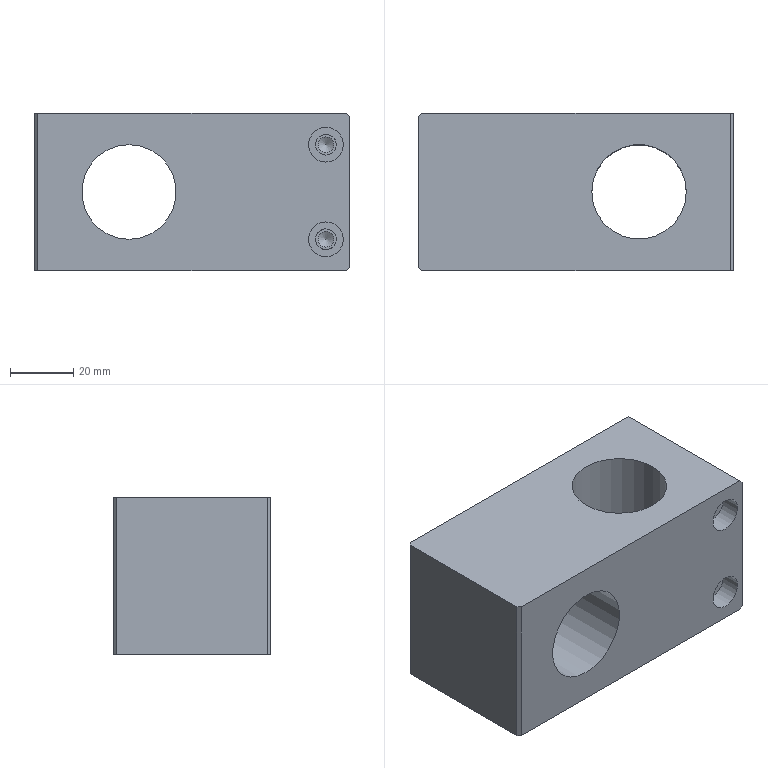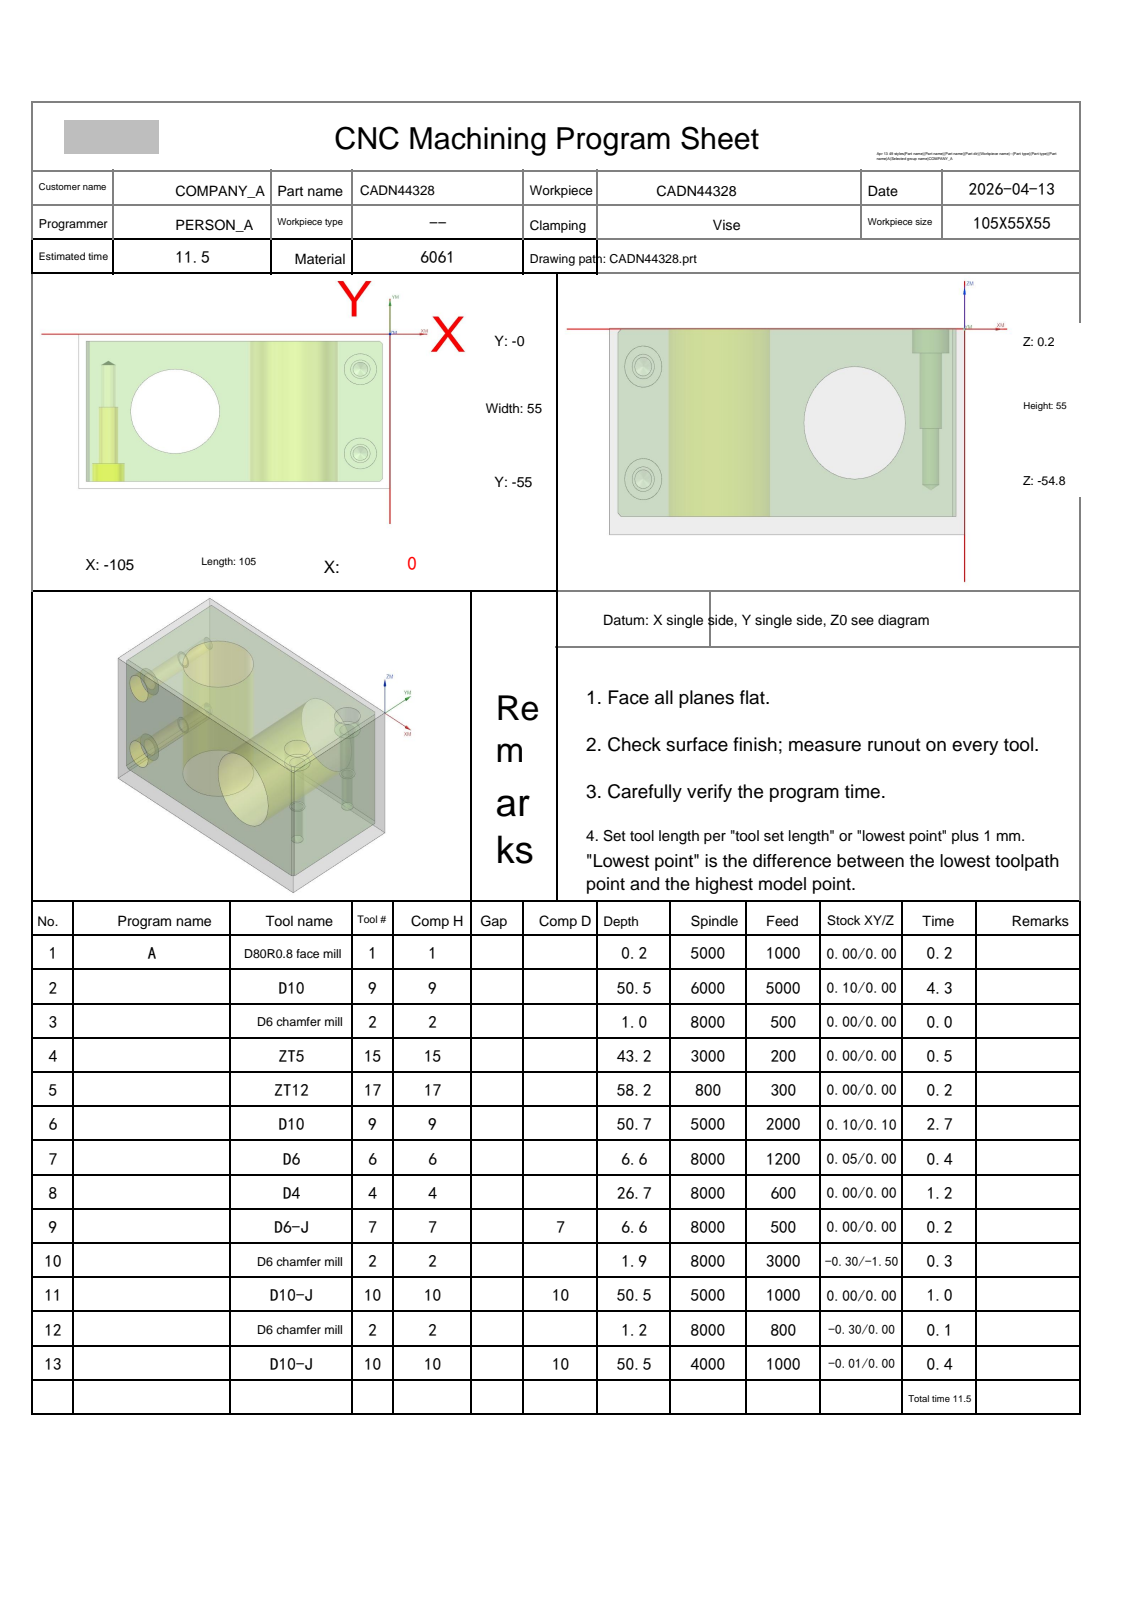NC program | NX | posted by the shop | part box 100 x 50 x 50 mm
Whole program, first 1102 of 1761 lines:
%
O0001
(Machine time: 14.12 MIN)
(===Total Tool:9===)
(T1=D80R0.8 face mill D=80. R=0.8 D- H01 Z=0.    )
(T9=D10 D=10. R=0. D- H09 Z=-50.5 )
(T2=D6 chamfer mill D=6. R=0. D- H02 Z=-1.7  )
(T15=ZT5 D=5. DR_a=118 D- H15 Z=-43.  )
(T17=ZT12 D=12. DR_a=118 D- H17 Z=-58.  )
(T6=D6 D=6. R=0. D- H06 Z=-6.4  )
(T4=D4 D=4. R=0. D- H04 Z=-26.5 )
(T7=D6-J D=6. R=0. D7 H07 Z=-6.4  )
(T10=D10-J D=10. R=0. D10 H10 Z=-50.3 )
G80 G90 G17 G49 G40
G91 G28 Z0
M01
N1 T01 M06
(D80R0.8 face mill D=80. R=0.8 H=01 ce=0.00 di=0.00)
G00 G90 G54 X42.5 Y-27.5 M03 S5000
G43 H01 Z20.
M08
Z2.
G01 Z0.0 F1000.
X37.5
X-142.5
X-147.5
Z2.
G00 Z20.
G91 G28 Z0.0
M05
M09
G91 G28 Z0.0
M01
N2 T09 M06
(D10 D=10. R=0. H=09 ce=0.10 di=0.00)
G00 G90 G54 X-53. Y-57.6 M03 S6000
G43 H09 Z20.
M08
Z.5
G01 X-102.5 Z.381 F5000.
G02 X-107.6 Y-52.5 Z.362 I0.0 J5.1
G01 Y-2.5 Z.242
G02 X-102.5 Y2.6 Z.223 I5.1 J0.0
G01 X-3.5 Z-.015
G02 X.106 Y1.106 Z-.024 I0.0 J-5.1
G01 X1.106 Y.106 Z-.028
G02 X2.6 Y-3.5 Z-.037 I-3.606 J-3.606
G01 Y-51.5 Z-.152
G02 X1.106 Y-55.106 Z-.162 I-5.1 J0.0
G01 X.106 Y-56.106 Z-.165
G02 X-3.5 Y-57.6 Z-.175 I-3.606 J3.606
G01 X-102.5 Z-.412
G02 X-107.6 Y-52.5 Z-.432 I0.0 J5.1
G01 Y-2.5 Z-.552
G02 X-102.5 Y2.6 Z-.571 I5.1 J0.0
G01 X-3.5 Z-.808
G02 X.106 Y1.106 Z-.818 I0.0 J-5.1
G01 X1.106 Y.106 Z-.821
G02 X2.6 Y-3.5 Z-.831 I-3.606 J-3.606
G01 Y-51.5 Z-.946
G02 X1.106 Y-55.106 Z-.956 I-5.1 J0.0
G01 X.106 Y-56.106 Z-.959
G02 X-3.5 Y-57.6 Z-.969 I-3.606 J3.606
G01 X-102.5 Z-1.206
G02 X-107.6 Y-52.5 Z-1.225 I0.0 J5.1
G01 Y-2.5 Z-1.345
G02 X-102.5 Y2.6 Z-1.365 I5.1 J0.0
G01 X-3.5 Z-1.602
G02 X.106 Y1.106 Z-1.612 I0.0 J-5.1
G01 X1.106 Y.106 Z-1.615
G02 X2.6 Y-3.5 Z-1.625 I-3.606 J-3.606
G01 Y-51.5 Z-1.74
G02 X1.106 Y-55.106 Z-1.75 I-5.1 J0.0
G01 X.106 Y-56.106 Z-1.753
G02 X-3.5 Y-57.6 Z-1.763 I-3.606 J3.606
G01 X-102.5 Z-2.
G02 X-107.6 Y-52.5 Z-2.019 I0.0 J5.1
G01 Y-2.5 Z-2.139
G02 X-102.5 Y2.6 Z-2.158 I5.1 J0.0
G01 X-3.5 Z-2.396
G02 X.106 Y1.106 Z-2.405 I0.0 J-5.1
G01 X1.106 Y.106 Z-2.409
G02 X2.6 Y-3.5 Z-2.418 I-3.606 J-3.606
G01 Y-51.5 Z-2.534
G02 X1.106 Y-55.106 Z-2.543 I-5.1 J0.0
G01 X.106 Y-56.106 Z-2.547
G02 X-3.5 Y-57.6 Z-2.556 I-3.606 J3.606
G01 X-102.5 Z-2.794
G02 X-107.6 Y-52.5 Z-2.813 I0.0 J5.1
G01 Y-2.5 Z-2.933
G02 X-102.5 Y2.6 Z-2.952 I5.1 J0.0
G01 X-3.5 Z-3.19
G02 X.106 Y1.106 Z-3.199 I0.0 J-5.1
G01 X1.106 Y.106 Z-3.203
G02 X2.6 Y-3.5 Z-3.212 I-3.606 J-3.606
G01 Y-51.5 Z-3.327
G02 X1.106 Y-55.106 Z-3.337 I-5.1 J0.0
G01 X.106 Y-56.106 Z-3.34
G02 X-3.5 Y-57.6 Z-3.35 I-3.606 J3.606
G01 X-102.5 Z-3.587
G02 X-107.6 Y-52.5 Z-3.607 I0.0 J5.1
G01 Y-2.5 Z-3.727
G02 X-102.5 Y2.6 Z-3.746 I5.1 J0.0
G01 X-3.5 Z-3.983
G02 X.106 Y1.106 Z-3.993 I0.0 J-5.1
G01 X1.106 Y.106 Z-3.996
G02 X2.6 Y-3.5 Z-4.006 I-3.606 J-3.606
G01 Y-51.5 Z-4.121
G02 X1.106 Y-55.106 Z-4.131 I-5.1 J0.0
G01 X.106 Y-56.106 Z-4.134
G02 X-3.5 Y-57.6 Z-4.144 I-3.606 J3.606
G01 X-102.5 Z-4.381
G02 X-107.6 Y-52.5 Z-4.4 I0.0 J5.1
G01 Y-2.5 Z-4.52
G02 X-102.5 Y2.6 Z-4.54 I5.1 J0.0
G01 X-3.5 Z-4.777
G02 X.106 Y1.106 Z-4.787 I0.0 J-5.1
G01 X1.106 Y.106 Z-4.79
G02 X2.6 Y-3.5 Z-4.8 I-3.606 J-3.606
G01 Y-51.5 Z-4.915
G02 X1.106 Y-55.106 Z-4.925 I-5.1 J0.0
G01 X.106 Y-56.106 Z-4.928
G02 X-3.5 Y-57.6 Z-4.938 I-3.606 J3.606
G01 X-102.5 Z-5.175
G02 X-107.6 Y-52.5 Z-5.194 I0.0 J5.1
G01 Y-2.5 Z-5.314
G02 X-102.5 Y2.6 Z-5.333 I5.1 J0.0
G01 X-3.5 Z-5.571
G02 X.106 Y1.106 Z-5.58 I0.0 J-5.1
G01 X1.106 Y.106 Z-5.584
G02 X2.6 Y-3.5 Z-5.593 I-3.606 J-3.606
G01 Y-51.5 Z-5.709
G02 X1.106 Y-55.106 Z-5.718 I-5.1 J0.0
G01 X.106 Y-56.106 Z-5.722
G02 X-3.5 Y-57.6 Z-5.731 I-3.606 J3.606
G01 X-102.5 Z-5.969
G02 X-107.6 Y-52.5 Z-5.988 I0.0 J5.1
G01 Y-2.5 Z-6.108
G02 X-102.5 Y2.6 Z-6.127 I5.1 J0.0
G01 X-3.5 Z-6.365
G02 X.106 Y1.106 Z-6.374 I0.0 J-5.1
G01 X1.106 Y.106 Z-6.378
G02 X2.6 Y-3.5 Z-6.387 I-3.606 J-3.606
G01 Y-51.5 Z-6.502
G02 X1.106 Y-55.106 Z-6.512 I-5.1 J0.0
G01 X.106 Y-56.106 Z-6.515
G02 X-3.5 Y-57.6 Z-6.525 I-3.606 J3.606
G01 X-102.5 Z-6.762
G02 X-107.6 Y-52.5 Z-6.782 I0.0 J5.1
G01 Y-2.5 Z-6.902
G02 X-102.5 Y2.6 Z-6.921 I5.1 J0.0
G01 X-3.5 Z-7.158
G02 X.106 Y1.106 Z-7.168 I0.0 J-5.1
G01 X1.106 Y.106 Z-7.171
G02 X2.6 Y-3.5 Z-7.181 I-3.606 J-3.606
G01 Y-51.5 Z-7.296
G02 X1.106 Y-55.106 Z-7.306 I-5.1 J0.0
G01 X.106 Y-56.106 Z-7.309
G02 X-3.5 Y-57.6 Z-7.319 I-3.606 J3.606
G01 X-102.5 Z-7.556
G02 X-107.6 Y-52.5 Z-7.575 I0.0 J5.1
G01 Y-2.5 Z-7.695
G02 X-102.5 Y2.6 Z-7.715 I5.1 J0.0
G01 X-3.5 Z-7.952
G02 X.106 Y1.106 Z-7.962 I0.0 J-5.1
G01 X1.106 Y.106 Z-7.965
G02 X2.6 Y-3.5 Z-7.975 I-3.606 J-3.606
G01 Y-51.5 Z-8.09
G02 X1.106 Y-55.106 Z-8.1 I-5.1 J0.0
G01 X.106 Y-56.106 Z-8.103
G02 X-3.5 Y-57.6 Z-8.113 I-3.606 J3.606
G01 X-102.5 Z-8.35
G02 X-107.6 Y-52.5 Z-8.369 I0.0 J5.1
G01 Y-2.5 Z-8.489
G02 X-102.5 Y2.6 Z-8.508 I5.1 J0.0
G01 X-3.5 Z-8.746
G02 X.106 Y1.106 Z-8.755 I0.0 J-5.1
G01 X1.106 Y.106 Z-8.759
G02 X2.6 Y-3.5 Z-8.768 I-3.606 J-3.606
G01 Y-51.5 Z-8.884
G02 X1.106 Y-55.106 Z-8.893 I-5.1 J0.0
G01 X.106 Y-56.106 Z-8.897
G02 X-3.5 Y-57.6 Z-8.906 I-3.606 J3.606
G01 X-102.5 Z-9.144
G02 X-107.6 Y-52.5 Z-9.163 I0.0 J5.1
G01 Y-2.5 Z-9.283
G02 X-102.5 Y2.6 Z-9.302 I5.1 J0.0
G01 X-3.5 Z-9.54
G02 X.106 Y1.106 Z-9.549 I0.0 J-5.1
G01 X1.106 Y.106 Z-9.553
G02 X2.6 Y-3.5 Z-9.562 I-3.606 J-3.606
G01 Y-51.5 Z-9.677
G02 X1.106 Y-55.106 Z-9.687 I-5.1 J0.0
G01 X.106 Y-56.106 Z-9.69
G02 X-3.5 Y-57.6 Z-9.7 I-3.606 J3.606
G01 X-102.5 Z-9.937
G02 X-107.6 Y-52.5 Z-9.957 I0.0 J5.1
G01 Y-2.5 Z-10.077
G02 X-102.5 Y2.6 Z-10.096 I5.1 J0.0
G01 X-3.5 Z-10.333
G02 X.106 Y1.106 Z-10.343 I0.0 J-5.1
G01 X1.106 Y.106 Z-10.346
G02 X2.6 Y-3.5 Z-10.356 I-3.606 J-3.606
G01 Y-51.5 Z-10.471
G02 X1.106 Y-55.106 Z-10.481 I-5.1 J0.0
G01 X.106 Y-56.106 Z-10.484
G02 X-3.5 Y-57.6 Z-10.494 I-3.606 J3.606
G01 X-102.5 Z-10.731
G02 X-107.6 Y-52.5 Z-10.75 I0.0 J5.1
G01 Y-2.5 Z-10.87
G02 X-102.5 Y2.6 Z-10.89 I5.1 J0.0
G01 X-3.5 Z-11.127
G02 X.106 Y1.106 Z-11.137 I0.0 J-5.1
G01 X1.106 Y.106 Z-11.14
G02 X2.6 Y-3.5 Z-11.15 I-3.606 J-3.606
G01 Y-51.5 Z-11.265
G02 X1.106 Y-55.106 Z-11.275 I-5.1 J0.0
G01 X.106 Y-56.106 Z-11.278
G02 X-3.5 Y-57.6 Z-11.288 I-3.606 J3.606
G01 X-102.5 Z-11.525
G02 X-107.6 Y-52.5 Z-11.544 I0.0 J5.1
G01 Y-2.5 Z-11.664
G02 X-102.5 Y2.6 Z-11.683 I5.1 J0.0
G01 X-3.5 Z-11.921
G02 X.106 Y1.106 Z-11.93 I0.0 J-5.1
G01 X1.106 Y.106 Z-11.934
G02 X2.6 Y-3.5 Z-11.943 I-3.606 J-3.606
G01 Y-51.5 Z-12.059
G02 X1.106 Y-55.106 Z-12.068 I-5.1 J0.0
G01 X.106 Y-56.106 Z-12.072
G02 X-3.5 Y-57.6 Z-12.081 I-3.606 J3.606
G01 X-102.5 Z-12.319
G02 X-107.6 Y-52.5 Z-12.338 I0.0 J5.1
G01 Y-2.5 Z-12.458
G02 X-102.5 Y2.6 Z-12.477 I5.1 J0.0
G01 X-3.5 Z-12.715
G02 X.106 Y1.106 Z-12.724 I0.0 J-5.1
G01 X1.106 Y.106 Z-12.728
G02 X2.6 Y-3.5 Z-12.737 I-3.606 J-3.606
G01 Y-51.5 Z-12.852
G02 X1.106 Y-55.106 Z-12.862 I-5.1 J0.0
G01 X.106 Y-56.106 Z-12.865
G02 X-3.5 Y-57.6 Z-12.875 I-3.606 J3.606
G01 X-102.5 Z-13.112
G02 X-107.6 Y-52.5 Z-13.132 I0.0 J5.1
G01 Y-2.5 Z-13.252
G02 X-102.5 Y2.6 Z-13.271 I5.1 J0.0
G01 X-3.5 Z-13.508
G02 X.106 Y1.106 Z-13.518 I0.0 J-5.1
G01 X1.106 Y.106 Z-13.521
G02 X2.6 Y-3.5 Z-13.531 I-3.606 J-3.606
G01 Y-51.5 Z-13.646
G02 X1.106 Y-55.106 Z-13.656 I-5.1 J0.0
G01 X.106 Y-56.106 Z-13.659
G02 X-3.5 Y-57.6 Z-13.669 I-3.606 J3.606
G01 X-102.5 Z-13.906
G02 X-107.6 Y-52.5 Z-13.925 I0.0 J5.1
G01 Y-2.5 Z-14.045
G02 X-102.5 Y2.6 Z-14.065 I5.1 J0.0
G01 X-3.5 Z-14.302
G02 X.106 Y1.106 Z-14.312 I0.0 J-5.1
G01 X1.106 Y.106 Z-14.315
G02 X2.6 Y-3.5 Z-14.325 I-3.606 J-3.606
G01 Y-51.5 Z-14.44
G02 X1.106 Y-55.106 Z-14.45 I-5.1 J0.0
G01 X.106 Y-56.106 Z-14.453
G02 X-3.5 Y-57.6 Z-14.463 I-3.606 J3.606
G01 X-102.5 Z-14.7
G02 X-107.6 Y-52.5 Z-14.719 I0.0 J5.1
G01 Y-2.5 Z-14.839
G02 X-102.5 Y2.6 Z-14.858 I5.1 J0.0
G01 X-3.5 Z-15.096
G02 X.106 Y1.106 Z-15.105 I0.0 J-5.1
G01 X1.106 Y.106 Z-15.109
G02 X2.6 Y-3.5 Z-15.118 I-3.606 J-3.606
G01 Y-51.5 Z-15.234
G02 X1.106 Y-55.106 Z-15.243 I-5.1 J0.0
G01 X.106 Y-56.106 Z-15.247
G02 X-3.5 Y-57.6 Z-15.256 I-3.606 J3.606
G01 X-102.5 Z-15.494
G02 X-107.6 Y-52.5 Z-15.513 I0.0 J5.1
G01 Y-2.5 Z-15.633
G02 X-102.5 Y2.6 Z-15.652 I5.1 J0.0
G01 X-3.5 Z-15.89
G02 X.106 Y1.106 Z-15.899 I0.0 J-5.1
G01 X1.106 Y.106 Z-15.903
G02 X2.6 Y-3.5 Z-15.912 I-3.606 J-3.606
G01 Y-51.5 Z-16.027
G02 X1.106 Y-55.106 Z-16.037 I-5.1 J0.0
G01 X.106 Y-56.106 Z-16.04
G02 X-3.5 Y-57.6 Z-16.05 I-3.606 J3.606
G01 X-102.5 Z-16.287
G02 X-107.6 Y-52.5 Z-16.307 I0.0 J5.1
G01 Y-2.5 Z-16.427
G02 X-102.5 Y2.6 Z-16.446 I5.1 J0.0
G01 X-3.5 Z-16.683
G02 X.106 Y1.106 Z-16.693 I0.0 J-5.1
G01 X1.106 Y.106 Z-16.696
G02 X2.6 Y-3.5 Z-16.706 I-3.606 J-3.606
G01 Y-51.5 Z-16.821
G02 X1.106 Y-55.106 Z-16.831 I-5.1 J0.0
G01 X.106 Y-56.106 Z-16.834
G02 X-3.5 Y-57.6 Z-16.844 I-3.606 J3.606
G01 X-102.5 Z-17.081
G02 X-107.6 Y-52.5 Z-17.1 I0.0 J5.1
G01 Y-2.5 Z-17.22
G02 X-102.5 Y2.6 Z-17.24 I5.1 J0.0
G01 X-3.5 Z-17.477
G02 X.106 Y1.106 Z-17.487 I0.0 J-5.1
G01 X1.106 Y.106 Z-17.49
G02 X2.6 Y-3.5 Z-17.5 I-3.606 J-3.606
G01 Y-51.5 Z-17.615
G02 X1.106 Y-55.106 Z-17.625 I-5.1 J0.0
G01 X.106 Y-56.106 Z-17.628
G02 X-3.5 Y-57.6 Z-17.638 I-3.606 J3.606
G01 X-102.5 Z-17.875
G02 X-107.6 Y-52.5 Z-17.894 I0.0 J5.1
G01 Y-2.5 Z-18.014
G02 X-102.5 Y2.6 Z-18.033 I5.1 J0.0
G01 X-3.5 Z-18.271
G02 X.106 Y1.106 Z-18.28 I0.0 J-5.1
G01 X1.106 Y.106 Z-18.284
G02 X2.6 Y-3.5 Z-18.293 I-3.606 J-3.606
G01 Y-51.5 Z-18.409
G02 X1.106 Y-55.106 Z-18.418 I-5.1 J0.0
G01 X.106 Y-56.106 Z-18.422
G02 X-3.5 Y-57.6 Z-18.431 I-3.606 J3.606
G01 X-102.5 Z-18.669
G02 X-107.6 Y-52.5 Z-18.688 I0.0 J5.1
G01 Y-2.5 Z-18.808
G02 X-102.5 Y2.6 Z-18.827 I5.1 J0.0
G01 X-3.5 Z-19.065
G02 X.106 Y1.106 Z-19.074 I0.0 J-5.1
G01 X1.106 Y.106 Z-19.078
G02 X2.6 Y-3.5 Z-19.087 I-3.606 J-3.606
G01 Y-51.5 Z-19.202
G02 X1.106 Y-55.106 Z-19.212 I-5.1 J0.0
G01 X.106 Y-56.106 Z-19.215
G02 X-3.5 Y-57.6 Z-19.225 I-3.606 J3.606
G01 X-102.5 Z-19.462
G02 X-107.6 Y-52.5 Z-19.482 I0.0 J5.1
G01 Y-2.5 Z-19.602
G02 X-102.5 Y2.6 Z-19.621 I5.1 J0.0
G01 X-3.5 Z-19.858
G02 X.106 Y1.106 Z-19.868 I0.0 J-5.1
G01 X1.106 Y.106 Z-19.871
G02 X2.6 Y-3.5 Z-19.881 I-3.606 J-3.606
G01 Y-51.5 Z-19.996
G02 X1.106 Y-55.106 Z-20.006 I-5.1 J0.0
G01 X.106 Y-56.106 Z-20.009
G02 X-3.5 Y-57.6 Z-20.019 I-3.606 J3.606
G01 X-102.5 Z-20.256
G02 X-107.6 Y-52.5 Z-20.275 I0.0 J5.1
G01 Y-2.5 Z-20.395
G02 X-102.5 Y2.6 Z-20.415 I5.1 J0.0
G01 X-3.5 Z-20.652
G02 X.106 Y1.106 Z-20.662 I0.0 J-5.1
G01 X1.106 Y.106 Z-20.665
G02 X2.6 Y-3.5 Z-20.675 I-3.606 J-3.606
G01 Y-51.5 Z-20.79
G02 X1.106 Y-55.106 Z-20.8 I-5.1 J0.0
G01 X.106 Y-56.106 Z-20.803
G02 X-3.5 Y-57.6 Z-20.813 I-3.606 J3.606
G01 X-102.5 Z-21.05
G02 X-107.6 Y-52.5 Z-21.069 I0.0 J5.1
G01 Y-2.5 Z-21.189
G02 X-102.5 Y2.6 Z-21.208 I5.1 J0.0
G01 X-3.5 Z-21.446
G02 X.106 Y1.106 Z-21.455 I0.0 J-5.1
G01 X1.106 Y.106 Z-21.459
G02 X2.6 Y-3.5 Z-21.468 I-3.606 J-3.606
G01 Y-51.5 Z-21.584
G02 X1.106 Y-55.106 Z-21.593 I-5.1 J0.0
G01 X.106 Y-56.106 Z-21.597
G02 X-3.5 Y-57.6 Z-21.606 I-3.606 J3.606
G01 X-102.5 Z-21.844
G02 X-107.6 Y-52.5 Z-21.863 I0.0 J5.1
G01 Y-2.5 Z-21.983
G02 X-102.5 Y2.6 Z-22.002 I5.1 J0.0
G01 X-3.5 Z-22.24
G02 X.106 Y1.106 Z-22.249 I0.0 J-5.1
G01 X1.106 Y.106 Z-22.253
G02 X2.6 Y-3.5 Z-22.262 I-3.606 J-3.606
G01 Y-51.5 Z-22.377
G02 X1.106 Y-55.106 Z-22.387 I-5.1 J0.0
G01 X.106 Y-56.106 Z-22.39
G02 X-3.5 Y-57.6 Z-22.4 I-3.606 J3.606
G01 X-102.5 Z-22.637
G02 X-107.6 Y-52.5 Z-22.657 I0.0 J5.1
G01 Y-2.5 Z-22.777
G02 X-102.5 Y2.6 Z-22.796 I5.1 J0.0
G01 X-3.5 Z-23.033
G02 X.106 Y1.106 Z-23.043 I0.0 J-5.1
G01 X1.106 Y.106 Z-23.046
G02 X2.6 Y-3.5 Z-23.056 I-3.606 J-3.606
G01 Y-51.5 Z-23.171
G02 X1.106 Y-55.106 Z-23.181 I-5.1 J0.0
G01 X.106 Y-56.106 Z-23.184
G02 X-3.5 Y-57.6 Z-23.194 I-3.606 J3.606
G01 X-102.5 Z-23.431
G02 X-107.6 Y-52.5 Z-23.45 I0.0 J5.1
G01 Y-2.5 Z-23.57
G02 X-102.5 Y2.6 Z-23.59 I5.1 J0.0
G01 X-3.5 Z-23.827
G02 X.106 Y1.106 Z-23.837 I0.0 J-5.1
G01 X1.106 Y.106 Z-23.84
G02 X2.6 Y-3.5 Z-23.85 I-3.606 J-3.606
G01 Y-51.5 Z-23.965
G02 X1.106 Y-55.106 Z-23.975 I-5.1 J0.0
G01 X.106 Y-56.106 Z-23.978
G02 X-3.5 Y-57.6 Z-23.988 I-3.606 J3.606
G01 X-102.5 Z-24.225
G02 X-107.6 Y-52.5 Z-24.244 I0.0 J5.1
G01 Y-2.5 Z-24.364
G02 X-102.5 Y2.6 Z-24.383 I5.1 J0.0
G01 X-3.5 Z-24.621
G02 X.106 Y1.106 Z-24.63 I0.0 J-5.1
G01 X1.106 Y.106 Z-24.634
G02 X2.6 Y-3.5 Z-24.643 I-3.606 J-3.606
G01 Y-51.5 Z-24.759
G02 X1.106 Y-55.106 Z-24.768 I-5.1 J0.0
G01 X.106 Y-56.106 Z-24.772
G02 X-3.5 Y-57.6 Z-24.781 I-3.606 J3.606
G01 X-102.5 Z-25.019
G02 X-107.6 Y-52.5 Z-25.038 I0.0 J5.1
G01 Y-2.5 Z-25.158
G02 X-102.5 Y2.6 Z-25.177 I5.1 J0.0
G01 X-3.5 Z-25.415
G02 X.106 Y1.106 Z-25.424 I0.0 J-5.1
G01 X1.106 Y.106 Z-25.428
G02 X2.6 Y-3.5 Z-25.437 I-3.606 J-3.606
G01 Y-51.5 Z-25.552
G02 X1.106 Y-55.106 Z-25.562 I-5.1 J0.0
G01 X.106 Y-56.106 Z-25.565
G02 X-3.5 Y-57.6 Z-25.575 I-3.606 J3.606
G01 X-102.5 Z-25.812
G02 X-107.6 Y-52.5 Z-25.832 I0.0 J5.1
G01 Y-2.5 Z-25.952
G02 X-102.5 Y2.6 Z-25.971 I5.1 J0.0
G01 X-3.5 Z-26.208
G02 X.106 Y1.106 Z-26.218 I0.0 J-5.1
G01 X1.106 Y.106 Z-26.221
G02 X2.6 Y-3.5 Z-26.231 I-3.606 J-3.606
G01 Y-51.5 Z-26.346
G02 X1.106 Y-55.106 Z-26.356 I-5.1 J0.0
G01 X.106 Y-56.106 Z-26.359
G02 X-3.5 Y-57.6 Z-26.369 I-3.606 J3.606
G01 X-102.5 Z-26.606
G02 X-107.6 Y-52.5 Z-26.625 I0.0 J5.1
G01 Y-2.5 Z-26.745
G02 X-102.5 Y2.6 Z-26.765 I5.1 J0.0
G01 X-3.5 Z-27.002
G02 X.106 Y1.106 Z-27.012 I0.0 J-5.1
G01 X1.106 Y.106 Z-27.015
G02 X2.6 Y-3.5 Z-27.025 I-3.606 J-3.606
G01 Y-51.5 Z-27.14
G02 X1.106 Y-55.106 Z-27.15 I-5.1 J0.0
G01 X.106 Y-56.106 Z-27.153
G02 X-3.5 Y-57.6 Z-27.163 I-3.606 J3.606
G01 X-102.5 Z-27.4
G02 X-107.6 Y-52.5 Z-27.419 I0.0 J5.1
G01 Y-2.5 Z-27.539
G02 X-102.5 Y2.6 Z-27.558 I5.1 J0.0
G01 X-3.5 Z-27.796
G02 X.106 Y1.106 Z-27.805 I0.0 J-5.1
G01 X1.106 Y.106 Z-27.809
G02 X2.6 Y-3.5 Z-27.818 I-3.606 J-3.606
G01 Y-51.5 Z-27.934
G02 X1.106 Y-55.106 Z-27.943 I-5.1 J0.0
G01 X.106 Y-56.106 Z-27.947
G02 X-3.5 Y-57.6 Z-27.956 I-3.606 J3.606
G01 X-102.5 Z-28.194
G02 X-107.6 Y-52.5 Z-28.213 I0.0 J5.1
G01 Y-2.5 Z-28.333
G02 X-102.5 Y2.6 Z-28.352 I5.1 J0.0
G01 X-3.5 Z-28.59
G02 X.106 Y1.106 Z-28.599 I0.0 J-5.1
G01 X1.106 Y.106 Z-28.603
G02 X2.6 Y-3.5 Z-28.612 I-3.606 J-3.606
G01 Y-51.5 Z-28.727
G02 X1.106 Y-55.106 Z-28.737 I-5.1 J0.0
G01 X.106 Y-56.106 Z-28.74
G02 X-3.5 Y-57.6 Z-28.75 I-3.606 J3.606
G01 X-102.5 Z-28.987
G02 X-107.6 Y-52.5 Z-29.007 I0.0 J5.1
G01 Y-2.5 Z-29.127
G02 X-102.5 Y2.6 Z-29.146 I5.1 J0.0
G01 X-3.5 Z-29.383
G02 X.106 Y1.106 Z-29.393 I0.0 J-5.1
G01 X1.106 Y.106 Z-29.396
G02 X2.6 Y-3.5 Z-29.406 I-3.606 J-3.606
G01 Y-51.5 Z-29.521
G02 X1.106 Y-55.106 Z-29.531 I-5.1 J0.0
G01 X.106 Y-56.106 Z-29.534
G02 X-3.5 Y-57.6 Z-29.544 I-3.606 J3.606
G01 X-102.5 Z-29.781
G02 X-107.6 Y-52.5 Z-29.8 I0.0 J5.1
G01 Y-2.5 Z-29.92
G02 X-102.5 Y2.6 Z-29.94 I5.1 J0.0
G01 X-3.5 Z-30.177
G02 X.106 Y1.106 Z-30.187 I0.0 J-5.1
G01 X1.106 Y.106 Z-30.19
G02 X2.6 Y-3.5 Z-30.2 I-3.606 J-3.606
G01 Y-51.5 Z-30.315
G02 X1.106 Y-55.106 Z-30.325 I-5.1 J0.0
G01 X.106 Y-56.106 Z-30.328
G02 X-3.5 Y-57.6 Z-30.338 I-3.606 J3.606
G01 X-102.5 Z-30.575
G02 X-107.6 Y-52.5 Z-30.594 I0.0 J5.1
G01 Y-2.5 Z-30.714
G02 X-102.5 Y2.6 Z-30.733 I5.1 J0.0
G01 X-3.5 Z-30.971
G02 X.106 Y1.106 Z-30.98 I0.0 J-5.1
G01 X1.106 Y.106 Z-30.984
G02 X2.6 Y-3.5 Z-30.993 I-3.606 J-3.606
G01 Y-51.5 Z-31.109
G02 X1.106 Y-55.106 Z-31.118 I-5.1 J0.0
G01 X.106 Y-56.106 Z-31.122
G02 X-3.5 Y-57.6 Z-31.131 I-3.606 J3.606
G01 X-102.5 Z-31.369
G02 X-107.6 Y-52.5 Z-31.388 I0.0 J5.1
G01 Y-2.5 Z-31.508
G02 X-102.5 Y2.6 Z-31.527 I5.1 J0.0
G01 X-3.5 Z-31.765
G02 X.106 Y1.106 Z-31.774 I0.0 J-5.1
G01 X1.106 Y.106 Z-31.778
G02 X2.6 Y-3.5 Z-31.787 I-3.606 J-3.606
G01 Y-51.5 Z-31.902
G02 X1.106 Y-55.106 Z-31.912 I-5.1 J0.0
G01 X.106 Y-56.106 Z-31.915
G02 X-3.5 Y-57.6 Z-31.925 I-3.606 J3.606
G01 X-102.5 Z-32.162
G02 X-107.6 Y-52.5 Z-32.182 I0.0 J5.1
G01 Y-2.5 Z-32.302
G02 X-102.5 Y2.6 Z-32.321 I5.1 J0.0
G01 X-3.5 Z-32.558
G02 X.106 Y1.106 Z-32.568 I0.0 J-5.1
G01 X1.106 Y.106 Z-32.571
G02 X2.6 Y-3.5 Z-32.581 I-3.606 J-3.606
G01 Y-51.5 Z-32.696
G02 X1.106 Y-55.106 Z-32.706 I-5.1 J0.0
G01 X.106 Y-56.106 Z-32.709
G02 X-3.5 Y-57.6 Z-32.719 I-3.606 J3.606
G01 X-102.5 Z-32.956
G02 X-107.6 Y-52.5 Z-32.975 I0.0 J5.1
G01 Y-2.5 Z-33.095
G02 X-102.5 Y2.6 Z-33.115 I5.1 J0.0
G01 X-3.5 Z-33.352
G02 X.106 Y1.106 Z-33.362 I0.0 J-5.1
G01 X1.106 Y.106 Z-33.365
G02 X2.6 Y-3.5 Z-33.375 I-3.606 J-3.606
G01 Y-51.5 Z-33.49
G02 X1.106 Y-55.106 Z-33.5 I-5.1 J0.0
G01 X.106 Y-56.106 Z-33.503
G02 X-3.5 Y-57.6 Z-33.513 I-3.606 J3.606
G01 X-102.5 Z-33.75
G02 X-107.6 Y-52.5 Z-33.769 I0.0 J5.1
G01 Y-2.5 Z-33.889
G02 X-102.5 Y2.6 Z-33.908 I5.1 J0.0
G01 X-3.5 Z-34.146
G02 X.106 Y1.106 Z-34.155 I0.0 J-5.1
G01 X1.106 Y.106 Z-34.159
G02 X2.6 Y-3.5 Z-34.168 I-3.606 J-3.606
G01 Y-51.5 Z-34.284
G02 X1.106 Y-55.106 Z-34.293 I-5.1 J0.0
G01 X.106 Y-56.106 Z-34.297
G02 X-3.5 Y-57.6 Z-34.306 I-3.606 J3.606
G01 X-102.5 Z-34.544
G02 X-107.6 Y-52.5 Z-34.563 I0.0 J5.1
G01 Y-2.5 Z-34.683
G02 X-102.5 Y2.6 Z-34.702 I5.1 J0.0
G01 X-3.5 Z-34.94
G02 X.106 Y1.106 Z-34.949 I0.0 J-5.1
G01 X1.106 Y.106 Z-34.953
G02 X2.6 Y-3.5 Z-34.962 I-3.606 J-3.606
G01 Y-51.5 Z-35.077
G02 X1.106 Y-55.106 Z-35.087 I-5.1 J0.0
G01 X.106 Y-56.106 Z-35.09
G02 X-3.5 Y-57.6 Z-35.1 I-3.606 J3.606
G01 X-102.5 Z-35.337
G02 X-107.6 Y-52.5 Z-35.357 I0.0 J5.1
G01 Y-2.5 Z-35.477
G02 X-102.5 Y2.6 Z-35.496 I5.1 J0.0
G01 X-3.5 Z-35.733
G02 X.106 Y1.106 Z-35.743 I0.0 J-5.1
G01 X1.106 Y.106 Z-35.746
G02 X2.6 Y-3.5 Z-35.756 I-3.606 J-3.606
G01 Y-51.5 Z-35.871
G02 X1.106 Y-55.106 Z-35.881 I-5.1 J0.0
G01 X.106 Y-56.106 Z-35.884
G02 X-3.5 Y-57.6 Z-35.894 I-3.606 J3.606
G01 X-102.5 Z-36.131
G02 X-107.6 Y-52.5 Z-36.15 I0.0 J5.1
G01 Y-2.5 Z-36.27
G02 X-102.5 Y2.6 Z-36.29 I5.1 J0.0
G01 X-3.5 Z-36.527
G02 X.106 Y1.106 Z-36.537 I0.0 J-5.1
G01 X1.106 Y.106 Z-36.54
G02 X2.6 Y-3.5 Z-36.55 I-3.606 J-3.606
G01 Y-51.5 Z-36.665
G02 X1.106 Y-55.106 Z-36.675 I-5.1 J0.0
G01 X.106 Y-56.106 Z-36.678
G02 X-3.5 Y-57.6 Z-36.688 I-3.606 J3.606
G01 X-102.5 Z-36.925
G02 X-107.6 Y-52.5 Z-36.944 I0.0 J5.1
G01 Y-2.5 Z-37.064
G02 X-102.5 Y2.6 Z-37.083 I5.1 J0.0
G01 X-3.5 Z-37.321
G02 X.106 Y1.106 Z-37.33 I0.0 J-5.1
G01 X1.106 Y.106 Z-37.334
G02 X2.6 Y-3.5 Z-37.343 I-3.606 J-3.606
G01 Y-51.5 Z-37.459
G02 X1.106 Y-55.106 Z-37.468 I-5.1 J0.0
G01 X.106 Y-56.106 Z-37.472
G02 X-3.5 Y-57.6 Z-37.481 I-3.606 J3.606
G01 X-102.5 Z-37.719
G02 X-107.6 Y-52.5 Z-37.738 I0.0 J5.1
G01 Y-2.5 Z-37.858
G02 X-102.5 Y2.6 Z-37.877 I5.1 J0.0
G01 X-3.5 Z-38.115
G02 X.106 Y1.106 Z-38.124 I0.0 J-5.1
G01 X1.106 Y.106 Z-38.128
G02 X2.6 Y-3.5 Z-38.137 I-3.606 J-3.606
G01 Y-51.5 Z-38.252
G02 X1.106 Y-55.106 Z-38.262 I-5.1 J0.0
G01 X.106 Y-56.106 Z-38.265
G02 X-3.5 Y-57.6 Z-38.275 I-3.606 J3.606
G01 X-102.5 Z-38.512
G02 X-107.6 Y-52.5 Z-38.532 I0.0 J5.1
G01 Y-2.5 Z-38.652
G02 X-102.5 Y2.6 Z-38.671 I5.1 J0.0
G01 X-3.5 Z-38.908
G02 X.106 Y1.106 Z-38.918 I0.0 J-5.1
G01 X1.106 Y.106 Z-38.921
G02 X2.6 Y-3.5 Z-38.931 I-3.606 J-3.606
G01 Y-51.5 Z-39.046
G02 X1.106 Y-55.106 Z-39.056 I-5.1 J0.0
G01 X.106 Y-56.106 Z-39.059
G02 X-3.5 Y-57.6 Z-39.069 I-3.606 J3.606
G01 X-102.5 Z-39.306
G02 X-107.6 Y-52.5 Z-39.325 I0.0 J5.1
G01 Y-2.5 Z-39.445
G02 X-102.5 Y2.6 Z-39.465 I5.1 J0.0
G01 X-3.5 Z-39.702
G02 X.106 Y1.106 Z-39.712 I0.0 J-5.1
G01 X1.106 Y.106 Z-39.715
G02 X2.6 Y-3.5 Z-39.725 I-3.606 J-3.606
G01 Y-51.5 Z-39.84
G02 X1.106 Y-55.106 Z-39.85 I-5.1 J0.0
G01 X.106 Y-56.106 Z-39.853
G02 X-3.5 Y-57.6 Z-39.863 I-3.606 J3.606
G01 X-102.5 Z-40.1
G02 X-107.6 Y-52.5 Z-40.119 I0.0 J5.1
G01 Y-2.5 Z-40.239
G02 X-102.5 Y2.6 Z-40.258 I5.1 J0.0
G01 X-3.5 Z-40.496
G02 X.106 Y1.106 Z-40.505 I0.0 J-5.1
G01 X1.106 Y.106 Z-40.509
G02 X2.6 Y-3.5 Z-40.518 I-3.606 J-3.606
G01 Y-51.5 Z-40.634
G02 X1.106 Y-55.106 Z-40.643 I-5.1 J0.0
G01 X.106 Y-56.106 Z-40.647
G02 X-3.5 Y-57.6 Z-40.656 I-3.606 J3.606
G01 X-102.5 Z-40.894
G02 X-107.6 Y-52.5 Z-40.913 I0.0 J5.1
G01 Y-2.5 Z-41.033
G02 X-102.5 Y2.6 Z-41.052 I5.1 J0.0
G01 X-3.5 Z-41.29
G02 X.106 Y1.106 Z-41.299 I0.0 J-5.1
G01 X1.106 Y.106 Z-41.303
G02 X2.6 Y-3.5 Z-41.312 I-3.606 J-3.606
G01 Y-51.5 Z-41.427
G02 X1.106 Y-55.106 Z-41.437 I-5.1 J0.0
G01 X.106 Y-56.106 Z-41.44
G02 X-3.5 Y-57.6 Z-41.45 I-3.606 J3.606
G01 X-102.5 Z-41.687
G02 X-107.6 Y-52.5 Z-41.707 I0.0 J5.1
G01 Y-2.5 Z-41.827
G02 X-102.5 Y2.6 Z-41.846 I5.1 J0.0
G01 X-3.5 Z-42.083
G02 X.106 Y1.106 Z-42.093 I0.0 J-5.1
G01 X1.106 Y.106 Z-42.096
G02 X2.6 Y-3.5 Z-42.106 I-3.606 J-3.606
G01 Y-51.5 Z-42.221
G02 X1.106 Y-55.106 Z-42.231 I-5.1 J0.0
G01 X.106 Y-56.106 Z-42.234
G02 X-3.5 Y-57.6 Z-42.244 I-3.606 J3.606
G01 X-102.5 Z-42.481
G02 X-107.6 Y-52.5 Z-42.5 I0.0 J5.1
G01 Y-2.5 Z-42.62
G02 X-102.5 Y2.6 Z-42.64 I5.1 J0.0
G01 X-3.5 Z-42.877
G02 X.106 Y1.106 Z-42.887 I0.0 J-5.1
G01 X1.106 Y.106 Z-42.89
G02 X2.6 Y-3.5 Z-42.9 I-3.606 J-3.606
G01 Y-51.5 Z-43.015
G02 X1.106 Y-55.106 Z-43.025 I-5.1 J0.0
G01 X.106 Y-56.106 Z-43.028
G02 X-3.5 Y-57.6 Z-43.038 I-3.606 J3.606
G01 X-102.5 Z-43.275
G02 X-107.6 Y-52.5 Z-43.294 I0.0 J5.1
G01 Y-2.5 Z-43.414
G02 X-102.5 Y2.6 Z-43.433 I5.1 J0.0
G01 X-3.5 Z-43.671
G02 X.106 Y1.106 Z-43.68 I0.0 J-5.1
G01 X1.106 Y.106 Z-43.684
G02 X2.6 Y-3.5 Z-43.693 I-3.606 J-3.606
G01 Y-51.5 Z-43.809
G02 X1.106 Y-55.106 Z-43.818 I-5.1 J0.0
G01 X.106 Y-56.106 Z-43.822
G02 X-3.5 Y-57.6 Z-43.831 I-3.606 J3.606
G01 X-102.5 Z-44.069
G02 X-107.6 Y-52.5 Z-44.088 I0.0 J5.1
G01 Y-2.5 Z-44.208
G02 X-102.5 Y2.6 Z-44.227 I5.1 J0.0
G01 X-3.5 Z-44.465
G02 X.106 Y1.106 Z-44.474 I0.0 J-5.1
G01 X1.106 Y.106 Z-44.478
G02 X2.6 Y-3.5 Z-44.487 I-3.606 J-3.606
G01 Y-51.5 Z-44.602
G02 X1.106 Y-55.106 Z-44.612 I-5.1 J0.0
G01 X.106 Y-56.106 Z-44.615
G02 X-3.5 Y-57.6 Z-44.625 I-3.606 J3.606
G01 X-102.5 Z-44.862
G02 X-107.6 Y-52.5 Z-44.882 I0.0 J5.1
G01 Y-2.5 Z-45.002
G02 X-102.5 Y2.6 Z-45.021 I5.1 J0.0
G01 X-3.5 Z-45.258
G02 X.106 Y1.106 Z-45.268 I0.0 J-5.1
G01 X1.106 Y.106 Z-45.271
G02 X2.6 Y-3.5 Z-45.281 I-3.606 J-3.606
G01 Y-51.5 Z-45.396
G02 X1.106 Y-55.106 Z-45.406 I-5.1 J0.0
G01 X.106 Y-56.106 Z-45.409
G02 X-3.5 Y-57.6 Z-45.419 I-3.606 J3.606
G01 X-102.5 Z-45.656
G02 X-107.6 Y-52.5 Z-45.675 I0.0 J5.1
G01 Y-2.5 Z-45.795
G02 X-102.5 Y2.6 Z-45.815 I5.1 J0.0
G01 X-3.5 Z-46.052
G02 X.106 Y1.106 Z-46.062 I0.0 J-5.1
G01 X1.106 Y.106 Z-46.065
G02 X2.6 Y-3.5 Z-46.075 I-3.606 J-3.606
G01 Y-51.5 Z-46.19
G02 X1.106 Y-55.106 Z-46.2 I-5.1 J0.0
G01 X.106 Y-56.106 Z-46.203
G02 X-3.5 Y-57.6 Z-46.213 I-3.606 J3.606
G01 X-102.5 Z-46.45
G02 X-107.6 Y-52.5 Z-46.469 I0.0 J5.1
G01 Y-2.5 Z-46.589
G02 X-102.5 Y2.6 Z-46.608 I5.1 J0.0
G01 X-3.5 Z-46.846
G02 X.106 Y1.106 Z-46.855 I0.0 J-5.1
G01 X1.106 Y.106 Z-46.859
G02 X2.6 Y-3.5 Z-46.868 I-3.606 J-3.606
G01 Y-51.5 Z-46.984
G02 X1.106 Y-55.106 Z-46.993 I-5.1 J0.0
G01 X.106 Y-56.106 Z-46.997
G02 X-3.5 Y-57.6 Z-47.006 I-3.606 J3.606
G01 X-102.5 Z-47.244
G02 X-107.6 Y-52.5 Z-47.263 I0.0 J5.1
G01 Y-2.5 Z-47.383
G02 X-102.5 Y2.6 Z-47.402 I5.1 J0.0
G01 X-3.5 Z-47.64
G02 X.106 Y1.106 Z-47.649 I0.0 J-5.1
G01 X1.106 Y.106 Z-47.653
G02 X2.6 Y-3.5 Z-47.662 I-3.606 J-3.606
G01 Y-51.5 Z-47.777
G02 X1.106 Y-55.106 Z-47.787 I-5.1 J0.0
G01 X.106 Y-56.106 Z-47.79
G02 X-3.5 Y-57.6 Z-47.8 I-3.606 J3.606
G01 X-102.5 Z-48.037
G02 X-107.6 Y-52.5 Z-48.057 I0.0 J5.1
G01 Y-2.5 Z-48.177
G02 X-102.5 Y2.6 Z-48.196 I5.1 J0.0
G01 X-3.5 Z-48.433
G02 X.106 Y1.106 Z-48.443 I0.0 J-5.1
G01 X1.106 Y.106 Z-48.446
G02 X2.6 Y-3.5 Z-48.456 I-3.606 J-3.606
G01 Y-51.5 Z-48.571
G02 X1.106 Y-55.106 Z-48.581 I-5.1 J0.0
G01 X.106 Y-56.106 Z-48.584
G02 X-3.5 Y-57.6 Z-48.594 I-3.606 J3.606
G01 X-102.5 Z-48.831
G02 X-107.6 Y-52.5 Z-48.85 I0.0 J5.1
G01 Y-2.5 Z-48.97
G02 X-102.5 Y2.6 Z-48.99 I5.1 J0.0
G01 X-3.5 Z-49.227
G02 X.106 Y1.106 Z-49.237 I0.0 J-5.1
G01 X1.106 Y.106 Z-49.24
G02 X2.6 Y-3.5 Z-49.25 I-3.606 J-3.606
G01 Y-51.5 Z-49.365
G02 X1.106 Y-55.106 Z-49.375 I-5.1 J0.0
G01 X.106 Y-56.106 Z-49.378
G02 X-3.5 Y-57.6 Z-49.388 I-3.606 J3.606
G01 X-102.5 Z-49.625
G02 X-107.6 Y-52.5 Z-49.644 I0.0 J5.1
G01 Y-2.5 Z-49.764
G02 X-102.5 Y2.6 Z-49.783 I5.1 J0.0
G01 X-3.5 Z-50.021
G02 X.106 Y1.106 Z-50.03 I0.0 J-5.1
G01 X1.106 Y.106 Z-50.034
G02 X2.6 Y-3.5 Z-50.043 I-3.606 J-3.606
G01 Y-51.5 Z-50.159
G02 X1.106 Y-55.106 Z-50.168 I-5.1 J0.0
G01 X.106 Y-56.106 Z-50.172
G02 X-3.5 Y-57.6 Z-50.181 I-3.606 J3.606
G01 X-53. Z-50.3
X-102.5
G02 X-107.6 Y-52.5 I0.0 J5.1
G01 Y-2.5
G02 X-102.5 Y2.6 I5.1 J0.0
G01 X-3.5
G02 X.106 Y1.106 I0.0 J-5.1
G01 X1.106 Y.106
G02 X2.6 Y-3.5 I-3.606 J-3.606
G01 Y-51.5
G02 X1.106 Y-55.106 I-5.1 J0.0
G01 X.106 Y-56.106
G02 X-3.5 Y-57.6 I-3.606 J3.606
G01 X-53.
X-53.5
Z-49.3
G00 Z20.
G91 G28 Z0.0
M05
M09
G91 G28 Z0.0
M01
N3 T02 M06
(D6 chamfer mill D=6. R=0. H=02 ce=0.00 di=0.00)
G00 G90 G54 X-10. Y-42.5 M03 S8000
G43 H02 Z20.
M08
G98 G81 X-10. Y-42.5 Z-.8 R1. F500.
Y-12.5
X-72.5 Y-27.5
G80
G00 Z20.
G91 G28 Z0.0
M05
M09
G91 G28 Z0.0
M01
N4 T15 M06
(ZT5 D=5. DR_a=118 H=15)
G00 G90 G54 X-10. Y-42.5 M03 S3000
G43 H15 Z20.
M08
G98 G83 X-10. Y-42.5 Z-43.002 R1. F200. Q2.
Y-12.5
G80
G00 Z20.
G91 G28 Z0.0
M05
M09
G91 G28 Z0.0
M01
N5 T17 M06
(ZT12 D=12. DR_a=118 H=17)
G00 G90 G54 X-72.5 Y-27.5 M03 S800
G43 H17 Z20.
M08
G98 G83 X-72.5 Y-27.5 Z-58. R1. F300. Q3.
G80
G00 Z20.
G91 G28 Z0.0
M05
M09
G91 G28 Z0.0
M01
N6 T09 M06
(D10 D=10. R=0. H=09 ce=0.10 di=0.10)
G00 G90 G54 X-63.229 Y-30.924 M03 S5000
G43 H09 Z20.
M08
Z1.
G01 X-62.957 Y-30.244 Z.962 F2000.
X-62.6 Y-28.271 Z.857
Y-26.729 Z.776
X-62.957 Y-24.756 Z.671
X-63.702 Y-22.896 Z.566
X-64.806 Y-21.223 Z.461
X-66.223 Y-19.806 Z.356
X-67.896 Y-18.702 Z.251
X-69.756 Y-17.957 Z.145
X-71.729 Y-17.6 Z.04
X-72.5 Z0.0
G03 X-82.4 Y-27.5 Z-.149 I0.0 J-9.9
X-72.5 Y-37.4 Z-.297 I9.9 J0.0
X-62.6 Y-27.5 Z-.446 I0.0 J9.9
X-72.5 Y-17.6 Z-.594 I-9.9 J0.0
X-82.4 Y-27.5 Z-.743 I0.0 J-9.9
X-72.5 Y-37.4 Z-.891 I9.9 J0.0
X-62.6 Y-27.5 Z-1.04 I0.0 J9.9
X-72.5 Y-17.6 Z-1.188 I-9.9 J0.0
X-82.4 Y-27.5 Z-1.337 I0.0 J-9.9
X-72.5 Y-37.4 Z-1.485 I9.9 J0.0
X-62.6 Y-27.5 Z-1.634 I0.0 J9.9
X-72.5 Y-17.6 Z-1.782 I-9.9 J0.0
X-82.4 Y-27.5 Z-1.931 I0.0 J-9.9
X-72.5 Y-37.4 Z-2.079 I9.9 J0.0
X-62.6 Y-27.5 Z-2.228 I0.0 J9.9
X-72.5 Y-17.6 Z-2.376 I-9.9 J0.0
X-82.4 Y-27.5 Z-2.525 I0.0 J-9.9
X-72.5 Y-37.4 Z-2.674 I9.9 J0.0
X-62.6 Y-27.5 Z-2.822 I0.0 J9.9
X-72.5 Y-17.6 Z-2.971 I-9.9 J0.0
X-82.4 Y-27.5 Z-3.119 I0.0 J-9.9
X-72.5 Y-37.4 Z-3.268 I9.9 J0.0
X-62.6 Y-27.5 Z-3.416 I0.0 J9.9
X-72.5 Y-17.6 Z-3.565 I-9.9 J0.0
X-82.4 Y-27.5 Z-3.713 I0.0 J-9.9
X-72.5 Y-37.4 Z-3.862 I9.9 J0.0
X-62.6 Y-27.5 Z-4.01 I0.0 J9.9
X-72.5 Y-17.6 Z-4.159 I-9.9 J0.0
X-82.4 Y-27.5 Z-4.307 I0.0 J-9.9
X-72.5 Y-37.4 Z-4.456 I9.9 J0.0
X-62.6 Y-27.5 Z-4.604 I0.0 J9.9
X-72.5 Y-17.6 Z-4.753 I-9.9 J0.0
X-82.4 Y-27.5 Z-4.901 I0.0 J-9.9
X-72.5 Y-37.4 Z-5.05 I9.9 J0.0
X-62.6 Y-27.5 Z-5.199 I0.0 J9.9
X-72.5 Y-17.6 Z-5.347 I-9.9 J0.0
X-82.4 Y-27.5 Z-5.496 I0.0 J-9.9
X-72.5 Y-37.4 Z-5.644 I9.9 J0.0
X-62.6 Y-27.5 Z-5.793 I0.0 J9.9
X-72.5 Y-17.6 Z-5.941 I-9.9 J0.0
X-82.4 Y-27.5 Z-6.09 I0.0 J-9.9
X-72.5 Y-37.4 Z-6.238 I9.9 J0.0
X-62.6 Y-27.5 Z-6.387 I0.0 J9.9
X-72.5 Y-17.6 Z-6.535 I-9.9 J0.0
X-82.4 Y-27.5 Z-6.684 I0.0 J-9.9
X-72.5 Y-37.4 Z-6.832 I9.9 J0.0
X-62.6 Y-27.5 Z-6.981 I0.0 J9.9
X-72.5 Y-17.6 Z-7.129 I-9.9 J0.0
X-82.4 Y-27.5 Z-7.278 I0.0 J-9.9
X-72.5 Y-37.4 Z-7.426 I9.9 J0.0
X-62.6 Y-27.5 Z-7.575 I0.0 J9.9
X-72.5 Y-17.6 Z-7.724 I-9.9 J0.0
X-82.4 Y-27.5 Z-7.872 I0.0 J-9.9
X-72.5 Y-37.4 Z-8.021 I9.9 J0.0
X-62.6 Y-27.5 Z-8.169 I0.0 J9.9
X-72.5 Y-17.6 Z-8.318 I-9.9 J0.0
X-82.4 Y-27.5 Z-8.466 I0.0 J-9.9
X-72.5 Y-37.4 Z-8.615 I9.9 J0.0
X-62.6 Y-27.5 Z-8.763 I0.0 J9.9
X-72.5 Y-17.6 Z-8.912 I-9.9 J0.0
X-82.4 Y-27.5 Z-9.06 I0.0 J-9.9
X-72.5 Y-37.4 Z-9.209 I9.9 J0.0
X-62.6 Y-27.5 Z-9.357 I0.0 J9.9
X-72.5 Y-17.6 Z-9.506 I-9.9 J0.0
X-82.4 Y-27.5 Z-9.654 I0.0 J-9.9
X-72.5 Y-37.4 Z-9.803 I9.9 J0.0
X-62.6 Y-27.5 Z-9.951 I0.0 J9.9
X-72.5 Y-17.6 Z-10.1 I-9.9 J0.0
X-82.4 Y-27.5 Z-10.249 I0.0 J-9.9
X-72.5 Y-37.4 Z-10.397 I9.9 J0.0
X-62.6 Y-27.5 Z-10.546 I0.0 J9.9
X-72.5 Y-17.6 Z-10.694 I-9.9 J0.0
X-82.4 Y-27.5 Z-10.843 I0.0 J-9.9
X-72.5 Y-37.4 Z-10.991 I9.9 J0.0
X-62.6 Y-27.5 Z-11.14 I0.0 J9.9
X-72.5 Y-17.6 Z-11.288 I-9.9 J0.0
X-82.4 Y-27.5 Z-11.437 I0.0 J-9.9
X-72.5 Y-37.4 Z-11.585 I9.9 J0.0
X-62.6 Y-27.5 Z-11.734 I0.0 J9.9
X-72.5 Y-17.6 Z-11.882 I-9.9 J0.0
X-82.4 Y-27.5 Z-12.031 I0.0 J-9.9
X-72.5 Y-37.4 Z-12.179 I9.9 J0.0
X-62.6 Y-27.5 Z-12.328 I0.0 J9.9
X-72.5 Y-17.6 Z-12.476 I-9.9 J0.0
X-82.4 Y-27.5 Z-12.625 I0.0 J-9.9
X-72.5 Y-37.4 Z-12.774 I9.9 J0.0
X-62.6 Y-27.5 Z-12.922 I0.0 J9.9
X-72.5 Y-17.6 Z-13.071 I-9.9 J0.0
X-82.4 Y-27.5 Z-13.219 I0.0 J-9.9
X-72.5 Y-37.4 Z-13.368 I9.9 J0.0
X-62.6 Y-27.5 Z-13.516 I0.0 J9.9
X-72.5 Y-17.6 Z-13.665 I-9.9 J0.0
X-82.4 Y-27.5 Z-13.813 I0.0 J-9.9
X-72.5 Y-37.4 Z-13.962 I9.9 J0.0
X-62.6 Y-27.5 Z-14.11 I0.0 J9.9
X-72.5 Y-17.6 Z-14.259 I-9.9 J0.0
X-82.4 Y-27.5 Z-14.407 I0.0 J-9.9
X-72.5 Y-37.4 Z-14.556 I9.9 J0.0
X-62.6 Y-27.5 Z-14.704 I0.0 J9.9
X-72.5 Y-17.6 Z-14.853 I-9.9 J0.0
X-82.4 Y-27.5 Z-15.001 I0.0 J-9.9
X-72.5 Y-37.4 Z-15.15 I9.9 J0.0
X-62.6 Y-27.5 Z-15.299 I0.0 J9.9
X-72.5 Y-17.6 Z-15.447 I-9.9 J0.0
X-82.4 Y-27.5 Z-15.596 I0.0 J-9.9
X-72.5 Y-37.4 Z-15.744 I9.9 J0.0
X-62.6 Y-27.5 Z-15.893 I0.0 J9.9
X-72.5 Y-17.6 Z-16.041 I-9.9 J0.0
X-82.4 Y-27.5 Z-16.19 I0.0 J-9.9
X-72.5 Y-37.4 Z-16.338 I9.9 J0.0
X-62.6 Y-27.5 Z-16.487 I0.0 J9.9
X-72.5 Y-17.6 Z-16.635 I-9.9 J0.0
X-82.4 Y-27.5 Z-16.784 I0.0 J-9.9
X-72.5 Y-37.4 Z-16.932 I9.9 J0.0
X-62.6 Y-27.5 Z-17.081 I0.0 J9.9
X-72.5 Y-17.6 Z-17.229 I-9.9 J0.0
X-82.4 Y-27.5 Z-17.378 I0.0 J-9.9
X-72.5 Y-37.4 Z-17.526 I9.9 J0.0
X-62.6 Y-27.5 Z-17.675 I0.0 J9.9
X-72.5 Y-17.6 Z-17.824 I-9.9 J0.0
X-82.4 Y-27.5 Z-17.972 I0.0 J-9.9
X-72.5 Y-37.4 Z-18.121 I9.9 J0.0
X-62.6 Y-27.5 Z-18.269 I0.0 J9.9
X-72.5 Y-17.6 Z-18.418 I-9.9 J0.0
X-82.4 Y-27.5 Z-18.566 I0.0 J-9.9
X-72.5 Y-37.4 Z-18.715 I9.9 J0.0
X-62.6 Y-27.5 Z-18.863 I0.0 J9.9
X-72.5 Y-17.6 Z-19.012 I-9.9 J0.0
X-82.4 Y-27.5 Z-19.16 I0.0 J-9.9
X-72.5 Y-37.4 Z-19.309 I9.9 J0.0
X-62.6 Y-27.5 Z-19.457 I0.0 J9.9
X-72.5 Y-17.6 Z-19.606 I-9.9 J0.0
X-82.4 Y-27.5 Z-19.754 I0.0 J-9.9
X-72.5 Y-37.4 Z-19.903 I9.9 J0.0
X-62.6 Y-27.5 Z-20.051 I0.0 J9.9
X-72.5 Y-17.6 Z-20.2 I-9.9 J0.0
X-82.4 Y-27.5 Z-20.349 I0.0 J-9.9
X-72.5 Y-37.4 Z-20.497 I9.9 J0.0
X-62.6 Y-27.5 Z-20.646 I0.0 J9.9
X-72.5 Y-17.6 Z-20.794 I-9.9 J0.0
X-82.4 Y-27.5 Z-20.943 I0.0 J-9.9
X-72.5 Y-37.4 Z-21.091 I9.9 J0.0
X-62.6 Y-27.5 Z-21.24 I0.0 J9.9
X-72.5 Y-17.6 Z-21.388 I-9.9 J0.0
X-82.4 Y-27.5 Z-21.537 I0.0 J-9.9
X-72.5 Y-37.4 Z-21.685 I9.9 J0.0
X-62.6 Y-27.5 Z-21.834 I0.0 J9.9
X-72.5 Y-17.6 Z-21.982 I-9.9 J0.0
X-82.4 Y-27.5 Z-22.131 I0.0 J-9.9
X-72.5 Y-37.4 Z-22.279 I9.9 J0.0
X-62.6 Y-27.5 Z-22.428 I0.0 J9.9
X-72.5 Y-17.6 Z-22.576 I-9.9 J0.0
X-82.4 Y-27.5 Z-22.725 I0.0 J-9.9
X-72.5 Y-37.4 Z-22.874 I9.9 J0.0
X-62.6 Y-27.5 Z-23.022 I0.0 J9.9
X-72.5 Y-17.6 Z-23.171 I-9.9 J0.0
X-82.4 Y-27.5 Z-23.319 I0.0 J-9.9
X-72.5 Y-37.4 Z-23.468 I9.9 J0.0
X-62.6 Y-27.5 Z-23.616 I0.0 J9.9
X-72.5 Y-17.6 Z-23.765 I-9.9 J0.0
X-82.4 Y-27.5 Z-23.913 I0.0 J-9.9
X-72.5 Y-37.4 Z-24.062 I9.9 J0.0
X-62.6 Y-27.5 Z-24.21 I0.0 J9.9
X-72.5 Y-17.6 Z-24.359 I-9.9 J0.0
X-82.4 Y-27.5 Z-24.507 I0.0 J-9.9
X-72.5 Y-37.4 Z-24.656 I9.9 J0.0
X-62.6 Y-27.5 Z-24.804 I0.0 J9.9
X-72.5 Y-17.6 Z-24.953 I-9.9 J0.0
X-82.4 Y-27.5 Z-25.101 I0.0 J-9.9
X-72.5 Y-37.4 Z-25.25 I9.9 J0.0
X-62.6 Y-27.5 Z-25.399 I0.0 J9.9
X-72.5 Y-17.6 Z-25.547 I-9.9 J0.0
X-82.4 Y-27.5 Z-25.696 I0.0 J-9.9
X-72.5 Y-37.4 Z-25.844 I9.9 J0.0
X-62.6 Y-27.5 Z-25.993 I0.0 J9.9
X-72.5 Y-17.6 Z-26.141 I-9.9 J0.0
X-82.4 Y-27.5 Z-26.29 I0.0 J-9.9
X-72.5 Y-37.4 Z-26.438 I9.9 J0.0
X-62.6 Y-27.5 Z-26.587 I0.0 J9.9
X-72.5 Y-17.6 Z-26.735 I-9.9 J0.0
X-82.4 Y-27.5 Z-26.884 I0.0 J-9.9
X-72.5 Y-37.4 Z-27.032 I9.9 J0.0
X-62.6 Y-27.5 Z-27.181 I0.0 J9.9
X-72.5 Y-17.6 Z-27.329 I-9.9 J0.0
X-82.4 Y-27.5 Z-27.478 I0.0 J-9.9
X-72.5 Y-37.4 Z-27.626 I9.9 J0.0
X-62.6 Y-27.5 Z-27.775 I0.0 J9.9
X-72.5 Y-17.6 Z-27.924 I-9.9 J0.0
X-82.4 Y-27.5 Z-28.072 I0.0 J-9.9
X-72.5 Y-37.4 Z-28.221 I9.9 J0.0
X-62.6 Y-27.5 Z-28.369 I0.0 J9.9
X-72.5 Y-17.6 Z-28.518 I-9.9 J0.0
X-82.4 Y-27.5 Z-28.666 I0.0 J-9.9
X-72.5 Y-37.4 Z-28.815 I9.9 J0.0
X-62.6 Y-27.5 Z-28.963 I0.0 J9.9
X-72.5 Y-17.6 Z-29.112 I-9.9 J0.0
X-82.4 Y-27.5 Z-29.26 I0.0 J-9.9
X-72.5 Y-37.4 Z-29.409 I9.9 J0.0
X-62.6 Y-27.5 Z-29.557 I0.0 J9.9
X-72.5 Y-17.6 Z-29.706 I-9.9 J0.0
X-82.4 Y-27.5 Z-29.854 I0.0 J-9.9
X-72.5 Y-37.4 Z-30.003 I9.9 J0.0
X-62.6 Y-27.5 Z-30.151 I0.0 J9.9
X-72.5 Y-17.6 Z-30.3 I-9.9 J0.0
X-82.4 Y-27.5 Z-30.449 I0.0 J-9.9
X-72.5 Y-37.4 Z-30.597 I9.9 J0.0
X-62.6 Y-27.5 Z-30.746 I0.0 J9.9
X-72.5 Y-17.6 Z-30.894 I-9.9 J0.0
X-82.4 Y-27.5 Z-31.043 I0.0 J-9.9
X-72.5 Y-37.4 Z-31.191 I9.9 J0.0
X-62.6 Y-27.5 Z-31.34 I0.0 J9.9
X-72.5 Y-17.6 Z-31.488 I-9.9 J0.0
X-82.4 Y-27.5 Z-31.637 I0.0 J-9.9
X-72.5 Y-37.4 Z-31.785 I9.9 J0.0